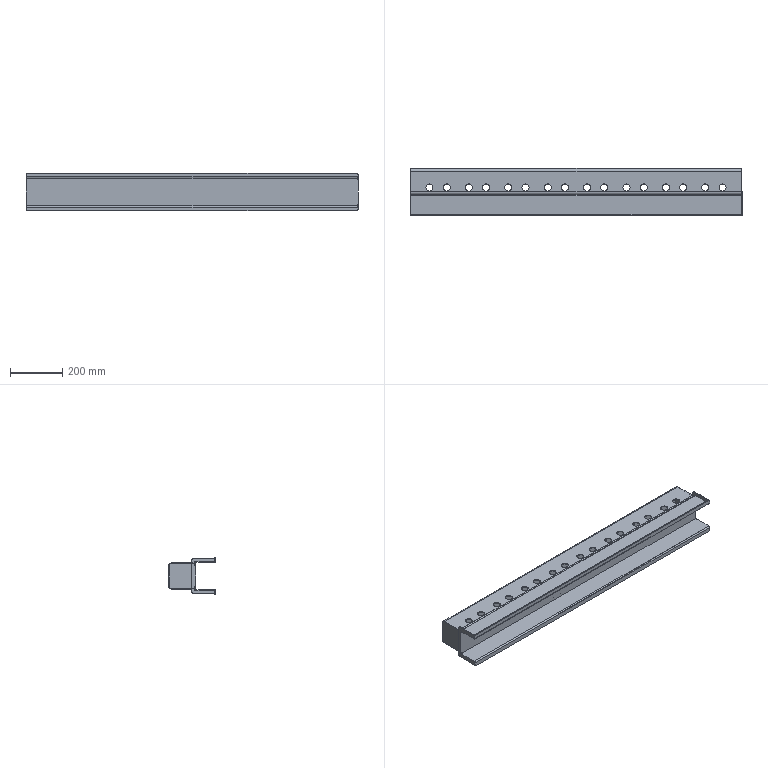Part | SolidWorks | features ICE 7, BaseBody 3, MoveCopyBody 1 | 1 solid | 154 faces | box 1272 x 180 x 145 mm | volume 2844306 mm3 | cylinder 106 | plane 48 | commonest cylinder face diameters 27.1 x64 63 x16 10 x8 20 x8 6 x6 14 x4